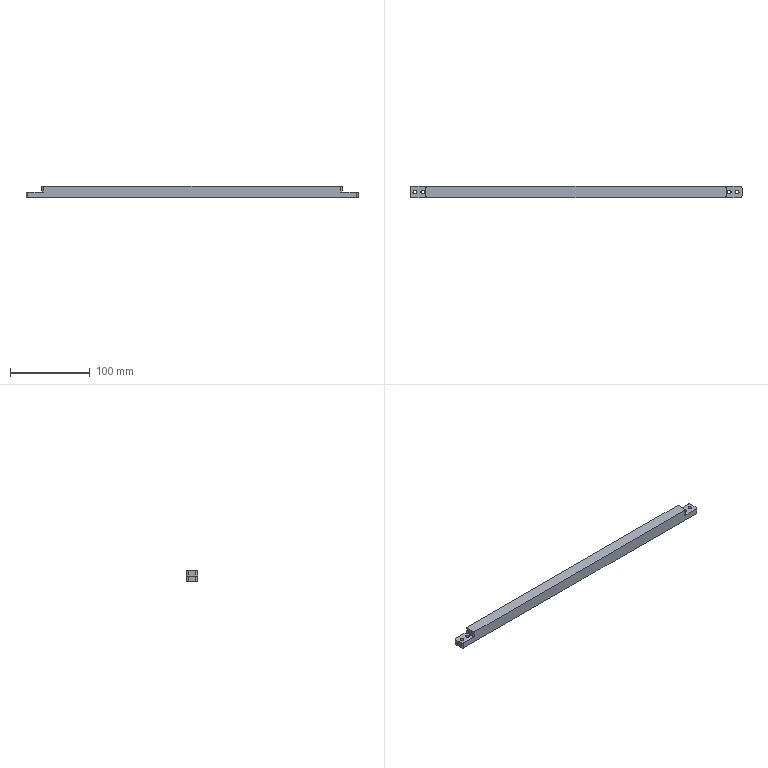Part | NX | 1 solid | 46 faces | box 417 x 14 x 15 mm | volume 81910 mm3 | cylinder 24 | plane 14 | cone 8 | commonest cylinder face diameters 2.459 x8 4 x8 4.5 x4 8 x4
STEP:
#1=CARTESIAN_POINT('',(-194.75,0.,-7.5));
#2=VERTEX_POINT('',#1);
#3=CARTESIAN_POINT('',(-192.5,0.,-7.5));
#4=DIRECTION('',(0.,0.,1.));
#5=DIRECTION('',(-1.,0.,0.));
#6=AXIS2_PLACEMENT_3D('',#3,#4,#5);
#7=CIRCLE('',#6,2.25);
#8=EDGE_CURVE('',#2,#2,#7,.T.);
#9=ORIENTED_EDGE('',*,*,#8,.T.);
#10=EDGE_LOOP('',(#9));
#11=FACE_BOUND('',#10,.T.);
#12=CARTESIAN_POINT('',(-194.75,0.,-10.5));
#13=VERTEX_POINT('',#12);
#14=CARTESIAN_POINT('',(-192.5,0.,-10.5));
#15=DIRECTION('',(0.,0.,1.));
#16=DIRECTION('',(-1.,0.,0.));
#17=AXIS2_PLACEMENT_3D('',#14,#15,#16);
#18=CIRCLE('',#17,2.25);
#19=EDGE_CURVE('',#13,#13,#18,.T.);
#20=ORIENTED_EDGE('',*,*,#19,.F.);
#21=EDGE_LOOP('',(#20));
#22=FACE_BOUND('',#21,.T.);
#23=CARTESIAN_POINT('',(-192.5,0.,-15.));
#24=DIRECTION('',(0.,0.,1.));
#25=DIRECTION('',(0.,-1.,0.));
#26=AXIS2_PLACEMENT_3D('',#23,#24,#25);
#27=CYLINDRICAL_SURFACE('',#26,2.25);
#28=ADVANCED_FACE('',(#11,#22),#27,.F.);
#29=CARTESIAN_POINT('',(-196.5,0.,-10.5));
#30=VERTEX_POINT('',#29);
#31=CARTESIAN_POINT('',(-192.5,0.,-10.5));
#32=DIRECTION('',(0.,0.,1.));
#33=DIRECTION('',(-1.,0.,0.));
#34=AXIS2_PLACEMENT_3D('',#31,#32,#33);
#35=CIRCLE('',#34,4.);
#36=EDGE_CURVE('',#30,#30,#35,.T.);
#37=ORIENTED_EDGE('',*,*,#36,.T.);
#38=EDGE_LOOP('',(#37));
#39=FACE_BOUND('',#38,.T.);
#40=CARTESIAN_POINT('',(-188.5,0.,-15.));
#41=VERTEX_POINT('',#40);
#42=CARTESIAN_POINT('',(-192.5,0.,-15.));
#43=DIRECTION('',(0.,0.,-1.));
#44=DIRECTION('',(1.,0.,0.));
#45=AXIS2_PLACEMENT_3D('',#42,#43,#44);
#46=CIRCLE('',#45,4.);
#47=EDGE_CURVE('',#41,#41,#46,.T.);
#48=ORIENTED_EDGE('',*,*,#47,.T.);
#49=EDGE_LOOP('',(#48));
#50=FACE_BOUND('',#49,.T.);
#51=CARTESIAN_POINT('',(-192.5,0.,-15.));
#52=DIRECTION('',(0.,0.,1.));
#53=DIRECTION('',(0.,-1.,0.));
#54=AXIS2_PLACEMENT_3D('',#51,#52,#53);
#55=CYLINDRICAL_SURFACE('',#54,4.);
#56=ADVANCED_FACE('',(#39,#50),#55,.F.);
#57=ORIENTED_EDGE('',*,*,#19,.T.);
#58=EDGE_LOOP('',(#57));
#59=FACE_BOUND('',#58,.T.);
#60=ORIENTED_EDGE('',*,*,#36,.F.);
#61=EDGE_LOOP('',(#60));
#62=FACE_BOUND('',#61,.T.);
#63=CARTESIAN_POINT('',(202.5,-2.25,-10.5));
#64=DIRECTION('',(0.,0.,1.));
#65=DIRECTION('',(0.,-1.,0.));
#66=AXIS2_PLACEMENT_3D('',#63,#64,#65);
#67=PLANE('',#66);
#68=ADVANCED_FACE('',(#59,#62),#67,.F.);
#69=CARTESIAN_POINT('',(-206.5,0.,-10.5));
#70=VERTEX_POINT('',#69);
#71=CARTESIAN_POINT('',(-202.5,0.,-10.5));
#72=DIRECTION('',(0.,0.,1.));
#73=DIRECTION('',(-1.,0.,0.));
#74=AXIS2_PLACEMENT_3D('',#71,#72,#73);
#75=CIRCLE('',#74,4.);
#76=EDGE_CURVE('',#70,#70,#75,.T.);
#77=ORIENTED_EDGE('',*,*,#76,.T.);
#78=EDGE_LOOP('',(#77));
#79=FACE_BOUND('',#78,.T.);
#80=CARTESIAN_POINT('',(-198.5,0.,-15.));
#81=VERTEX_POINT('',#80);
#82=CARTESIAN_POINT('',(-202.5,0.,-15.));
#83=DIRECTION('',(0.,0.,-1.));
#84=DIRECTION('',(1.,0.,0.));
#85=AXIS2_PLACEMENT_3D('',#82,#83,#84);
#86=CIRCLE('',#85,4.);
#87=EDGE_CURVE('',#81,#81,#86,.T.);
#88=ORIENTED_EDGE('',*,*,#87,.T.);
#89=EDGE_LOOP('',(#88));
#90=FACE_BOUND('',#89,.T.);
#91=CARTESIAN_POINT('',(-202.5,0.,-15.));
#92=DIRECTION('',(0.,0.,1.));
#93=DIRECTION('',(0.,-1.,0.));
#94=AXIS2_PLACEMENT_3D('',#91,#92,#93);
#95=CYLINDRICAL_SURFACE('',#94,4.);
#96=ADVANCED_FACE('',(#79,#90),#95,.F.);
#97=CARTESIAN_POINT('',(-206.5,-7.,-15.));
#98=VERTEX_POINT('',#97);
#99=CARTESIAN_POINT('',(-208.5,-5.,-15.));
#100=VERTEX_POINT('',#99);
#101=CARTESIAN_POINT('',(-206.5,-5.,-15.));
#102=DIRECTION('',(0.,0.,-1.));
#103=DIRECTION('',(1.,0.,0.));
#104=AXIS2_PLACEMENT_3D('',#101,#102,#103);
#105=CIRCLE('',#104,2.);
#106=EDGE_CURVE('',#98,#100,#105,.T.);
#107=ORIENTED_EDGE('',*,*,#106,.F.);
#108=CARTESIAN_POINT('',(-206.5,-7.,-7.5));
#109=VERTEX_POINT('',#108);
#110=CARTESIAN_POINT('',(-206.5,-7.,-11.25));
#111=DIRECTION('',(0.,0.,-1.));
#112=VECTOR('',#111,1000.);
#113=LINE('',#110,#112);
#114=EDGE_CURVE('',#109,#98,#113,.T.);
#115=ORIENTED_EDGE('',*,*,#114,.F.);
#116=CARTESIAN_POINT('',(-208.5,-5.,-7.5));
#117=VERTEX_POINT('',#116);
#118=CARTESIAN_POINT('',(-206.5,-5.,-7.5));
#119=DIRECTION('',(0.,0.,1.));
#120=DIRECTION('',(-1.,0.,0.));
#121=AXIS2_PLACEMENT_3D('',#118,#119,#120);
#122=CIRCLE('',#121,2.);
#123=EDGE_CURVE('',#117,#109,#122,.T.);
#124=ORIENTED_EDGE('',*,*,#123,.F.);
#125=CARTESIAN_POINT('',(-208.5,-5.,-11.25));
#126=DIRECTION('',(0.,0.,-1.));
#127=VECTOR('',#126,1000.);
#128=LINE('',#125,#127);
#129=EDGE_CURVE('',#117,#100,#128,.T.);
#130=ORIENTED_EDGE('',*,*,#129,.T.);
#131=EDGE_LOOP('',(#107,#115,#124,#130));
#132=FACE_BOUND('',#131,.T.);
#133=CARTESIAN_POINT('',(-206.5,-5.,-7.5));
#134=DIRECTION('',(0.,0.,-1.));
#135=DIRECTION('',(0.,-1.,0.));
#136=AXIS2_PLACEMENT_3D('',#133,#134,#135);
#137=CYLINDRICAL_SURFACE('',#136,2.);
#138=ADVANCED_FACE('',(#132),#137,.T.);
#139=CARTESIAN_POINT('',(-188.5,-5.,-7.5));
#140=VERTEX_POINT('',#139);
#141=CARTESIAN_POINT('',(-186.5,-7.,-7.5));
#142=VERTEX_POINT('',#141);
#143=CARTESIAN_POINT('',(-186.5,-5.,-7.5));
#144=DIRECTION('',(0.,0.,1.));
#145=DIRECTION('',(-1.,0.,0.));
#146=AXIS2_PLACEMENT_3D('',#143,#144,#145);
#147=CIRCLE('',#146,2.);
#148=EDGE_CURVE('',#140,#142,#147,.T.);
#149=ORIENTED_EDGE('',*,*,#148,.T.);
#150=CARTESIAN_POINT('',(-186.5,-7.,0.));
#151=VERTEX_POINT('',#150);
#152=CARTESIAN_POINT('',(-186.5,-7.,-3.75));
#153=DIRECTION('',(0.,0.,-1.));
#154=VECTOR('',#153,1000.);
#155=LINE('',#152,#154);
#156=EDGE_CURVE('',#151,#142,#155,.T.);
#157=ORIENTED_EDGE('',*,*,#156,.F.);
#158=CARTESIAN_POINT('',(-188.5,-5.,0.));
#159=VERTEX_POINT('',#158);
#160=CARTESIAN_POINT('',(-186.5,-5.,0.));
#161=DIRECTION('',(0.,0.,-1.));
#162=DIRECTION('',(1.,0.,0.));
#163=AXIS2_PLACEMENT_3D('',#160,#161,#162);
#164=CIRCLE('',#163,2.);
#165=EDGE_CURVE('',#151,#159,#164,.T.);
#166=ORIENTED_EDGE('',*,*,#165,.T.);
#167=CARTESIAN_POINT('',(-188.5,-5.,-3.75));
#168=DIRECTION('',(0.,0.,-1.));
#169=VECTOR('',#168,1000.);
#170=LINE('',#167,#169);
#171=EDGE_CURVE('',#159,#140,#170,.T.);
#172=ORIENTED_EDGE('',*,*,#171,.T.);
#173=EDGE_LOOP('',(#149,#157,#166,#172));
#174=FACE_BOUND('',#173,.T.);
#175=CARTESIAN_POINT('',(-186.5,-5.,-7.5));
#176=DIRECTION('',(0.,0.,-1.));
#177=DIRECTION('',(0.,-1.,0.));
#178=AXIS2_PLACEMENT_3D('',#175,#176,#177);
#179=CYLINDRICAL_SURFACE('',#178,2.);
#180=ADVANCED_FACE('',(#174),#179,.T.);
#181=CARTESIAN_POINT('',(-186.5,7.,-7.5));
#182=VERTEX_POINT('',#181);
#183=CARTESIAN_POINT('',(-188.5,5.,-7.5));
#184=VERTEX_POINT('',#183);
#185=CARTESIAN_POINT('',(-186.5,5.,-7.5));
#186=DIRECTION('',(0.,0.,1.));
#187=DIRECTION('',(-1.,0.,0.));
#188=AXIS2_PLACEMENT_3D('',#185,#186,#187);
#189=CIRCLE('',#188,2.);
#190=EDGE_CURVE('',#182,#184,#189,.T.);
#191=ORIENTED_EDGE('',*,*,#190,.T.);
#192=CARTESIAN_POINT('',(-188.5,5.,0.));
#193=VERTEX_POINT('',#192);
#194=CARTESIAN_POINT('',(-188.5,5.,-3.75));
#195=DIRECTION('',(0.,0.,-1.));
#196=VECTOR('',#195,1000.);
#197=LINE('',#194,#196);
#198=EDGE_CURVE('',#193,#184,#197,.T.);
#199=ORIENTED_EDGE('',*,*,#198,.F.);
#200=CARTESIAN_POINT('',(-186.5,7.,0.));
#201=VERTEX_POINT('',#200);
#202=CARTESIAN_POINT('',(-186.5,5.,0.));
#203=DIRECTION('',(0.,0.,-1.));
#204=DIRECTION('',(1.,0.,0.));
#205=AXIS2_PLACEMENT_3D('',#202,#203,#204);
#206=CIRCLE('',#205,2.);
#207=EDGE_CURVE('',#193,#201,#206,.T.);
#208=ORIENTED_EDGE('',*,*,#207,.T.);
#209=CARTESIAN_POINT('',(-186.5,7.,-3.75));
#210=DIRECTION('',(0.,0.,-1.));
#211=VECTOR('',#210,1000.);
#212=LINE('',#209,#211);
#213=EDGE_CURVE('',#201,#182,#212,.T.);
#214=ORIENTED_EDGE('',*,*,#213,.T.);
#215=EDGE_LOOP('',(#191,#199,#208,#214));
#216=FACE_BOUND('',#215,.T.);
#217=CARTESIAN_POINT('',(-186.5,5.,-7.5));
#218=DIRECTION('',(0.,0.,-1.));
#219=DIRECTION('',(-1.,0.,0.));
#220=AXIS2_PLACEMENT_3D('',#217,#218,#219);
#221=CYLINDRICAL_SURFACE('',#220,2.);
#222=ADVANCED_FACE('',(#216),#221,.T.);
#223=CARTESIAN_POINT('',(-208.5,5.,-15.));
#224=VERTEX_POINT('',#223);
#225=CARTESIAN_POINT('',(-206.5,7.,-15.));
#226=VERTEX_POINT('',#225);
#227=CARTESIAN_POINT('',(-206.5,5.,-15.));
#228=DIRECTION('',(0.,0.,-1.));
#229=DIRECTION('',(1.,0.,0.));
#230=AXIS2_PLACEMENT_3D('',#227,#228,#229);
#231=CIRCLE('',#230,2.);
#232=EDGE_CURVE('',#224,#226,#231,.T.);
#233=ORIENTED_EDGE('',*,*,#232,.F.);
#234=CARTESIAN_POINT('',(-208.5,5.,-7.5));
#235=VERTEX_POINT('',#234);
#236=CARTESIAN_POINT('',(-208.5,5.,-11.25));
#237=DIRECTION('',(0.,0.,-1.));
#238=VECTOR('',#237,1000.);
#239=LINE('',#236,#238);
#240=EDGE_CURVE('',#235,#224,#239,.T.);
#241=ORIENTED_EDGE('',*,*,#240,.F.);
#242=CARTESIAN_POINT('',(-206.5,7.,-7.5));
#243=VERTEX_POINT('',#242);
#244=CARTESIAN_POINT('',(-206.5,5.,-7.5));
#245=DIRECTION('',(0.,0.,1.));
#246=DIRECTION('',(-1.,0.,0.));
#247=AXIS2_PLACEMENT_3D('',#244,#245,#246);
#248=CIRCLE('',#247,2.);
#249=EDGE_CURVE('',#243,#235,#248,.T.);
#250=ORIENTED_EDGE('',*,*,#249,.F.);
#251=CARTESIAN_POINT('',(-206.5,7.,-11.25));
#252=DIRECTION('',(0.,0.,-1.));
#253=VECTOR('',#252,1000.);
#254=LINE('',#251,#253);
#255=EDGE_CURVE('',#243,#226,#254,.T.);
#256=ORIENTED_EDGE('',*,*,#255,.T.);
#257=EDGE_LOOP('',(#233,#241,#250,#256));
#258=FACE_BOUND('',#257,.T.);
#259=CARTESIAN_POINT('',(-206.5,5.,-7.5));
#260=DIRECTION('',(0.,0.,-1.));
#261=DIRECTION('',(-1.,0.,0.));
#262=AXIS2_PLACEMENT_3D('',#259,#260,#261);
#263=CYLINDRICAL_SURFACE('',#262,2.);
#264=ADVANCED_FACE('',(#258),#263,.T.);
#265=CARTESIAN_POINT('',(-174.23,0.,-15.));
#266=VERTEX_POINT('',#265);
#267=CARTESIAN_POINT('',(-173.,0.,-15.));
#268=DIRECTION('',(0.,0.,1.));
#269=DIRECTION('',(-1.,0.,0.));
#270=AXIS2_PLACEMENT_3D('',#267,#268,#269);
#271=CIRCLE('',#270,1.23);
#272=EDGE_CURVE('',#266,#266,#271,.T.);
#273=ORIENTED_EDGE('',*,*,#272,.T.);
#274=EDGE_LOOP('',(#273));
#275=FACE_BOUND('',#274,.T.);
#276=CARTESIAN_POINT('',(-124.23,0.,-15.));
#277=VERTEX_POINT('',#276);
#278=CARTESIAN_POINT('',(-123.,0.,-15.));
#279=DIRECTION('',(0.,0.,1.));
#280=DIRECTION('',(-1.,0.,0.));
#281=AXIS2_PLACEMENT_3D('',#278,#279,#280);
#282=CIRCLE('',#281,1.23);
#283=EDGE_CURVE('',#277,#277,#282,.T.);
#284=ORIENTED_EDGE('',*,*,#283,.T.);
#285=EDGE_LOOP('',(#284));
#286=FACE_BOUND('',#285,.T.);
#287=CARTESIAN_POINT('',(-74.23,0.,-15.));
#288=VERTEX_POINT('',#287);
#289=CARTESIAN_POINT('',(-73.,0.,-15.));
#290=DIRECTION('',(0.,0.,1.));
#291=DIRECTION('',(-1.,0.,0.));
#292=AXIS2_PLACEMENT_3D('',#289,#290,#291);
#293=CIRCLE('',#292,1.23);
#294=EDGE_CURVE('',#288,#288,#293,.T.);
#295=ORIENTED_EDGE('',*,*,#294,.T.);
#296=EDGE_LOOP('',(#295));
#297=FACE_BOUND('',#296,.T.);
#298=CARTESIAN_POINT('',(-24.23,0.,-15.));
#299=VERTEX_POINT('',#298);
#300=CARTESIAN_POINT('',(-23.,0.,-15.));
#301=DIRECTION('',(0.,0.,1.));
#302=DIRECTION('',(-1.,0.,0.));
#303=AXIS2_PLACEMENT_3D('',#300,#301,#302);
#304=CIRCLE('',#303,1.23);
#305=EDGE_CURVE('',#299,#299,#304,.T.);
#306=ORIENTED_EDGE('',*,*,#305,.T.);
#307=EDGE_LOOP('',(#306));
#308=FACE_BOUND('',#307,.T.);
#309=CARTESIAN_POINT('',(25.77,0.,-15.));
#310=VERTEX_POINT('',#309);
#311=CARTESIAN_POINT('',(27.,0.,-15.));
#312=DIRECTION('',(0.,0.,1.));
#313=DIRECTION('',(-1.,0.,0.));
#314=AXIS2_PLACEMENT_3D('',#311,#312,#313);
#315=CIRCLE('',#314,1.23);
#316=EDGE_CURVE('',#310,#310,#315,.T.);
#317=ORIENTED_EDGE('',*,*,#316,.T.);
#318=EDGE_LOOP('',(#317));
#319=FACE_BOUND('',#318,.T.);
#320=CARTESIAN_POINT('',(75.77,0.,-15.));
#321=VERTEX_POINT('',#320);
#322=CARTESIAN_POINT('',(77.,0.,-15.));
#323=DIRECTION('',(0.,0.,1.));
#324=DIRECTION('',(-1.,0.,0.));
#325=AXIS2_PLACEMENT_3D('',#322,#323,#324);
#326=CIRCLE('',#325,1.23);
#327=EDGE_CURVE('',#321,#321,#326,.T.);
#328=ORIENTED_EDGE('',*,*,#327,.T.);
#329=EDGE_LOOP('',(#328));
#330=FACE_BOUND('',#329,.T.);
#331=CARTESIAN_POINT('',(125.77,0.,-15.));
#332=VERTEX_POINT('',#331);
#333=CARTESIAN_POINT('',(127.,0.,-15.));
#334=DIRECTION('',(0.,0.,1.));
#335=DIRECTION('',(-1.,0.,0.));
#336=AXIS2_PLACEMENT_3D('',#333,#334,#335);
#337=CIRCLE('',#336,1.23);
#338=EDGE_CURVE('',#332,#332,#337,.T.);
#339=ORIENTED_EDGE('',*,*,#338,.T.);
#340=EDGE_LOOP('',(#339));
#341=FACE_BOUND('',#340,.T.);
#342=CARTESIAN_POINT('',(198.5,0.,-15.));
#343=VERTEX_POINT('',#342);
#344=CARTESIAN_POINT('',(202.5,0.,-15.));
#345=DIRECTION('',(0.,0.,1.));
#346=DIRECTION('',(-1.,0.,0.));
#347=AXIS2_PLACEMENT_3D('',#344,#345,#346);
#348=CIRCLE('',#347,4.);
#349=EDGE_CURVE('',#343,#343,#348,.T.);
#350=ORIENTED_EDGE('',*,*,#349,.T.);
#351=EDGE_LOOP('',(#350));
#352=FACE_BOUND('',#351,.T.);
#353=CARTESIAN_POINT('',(188.5,0.,-15.));
#354=VERTEX_POINT('',#353);
#355=CARTESIAN_POINT('',(192.5,0.,-15.));
#356=DIRECTION('',(0.,0.,1.));
#357=DIRECTION('',(-1.,0.,0.));
#358=AXIS2_PLACEMENT_3D('',#355,#356,#357);
#359=CIRCLE('',#358,4.);
#360=EDGE_CURVE('',#354,#354,#359,.T.);
#361=ORIENTED_EDGE('',*,*,#360,.T.);
#362=EDGE_LOOP('',(#361));
#363=FACE_BOUND('',#362,.T.);
#364=CARTESIAN_POINT('',(175.77,0.,-15.));
#365=VERTEX_POINT('',#364);
#366=CARTESIAN_POINT('',(177.,0.,-15.));
#367=DIRECTION('',(0.,0.,1.));
#368=DIRECTION('',(-1.,0.,0.));
#369=AXIS2_PLACEMENT_3D('',#366,#367,#368);
#370=CIRCLE('',#369,1.23);
#371=EDGE_CURVE('',#365,#365,#370,.T.);
#372=ORIENTED_EDGE('',*,*,#371,.T.);
#373=EDGE_LOOP('',(#372));
#374=FACE_BOUND('',#373,.T.);
#375=ORIENTED_EDGE('',*,*,#87,.F.);
#376=EDGE_LOOP('',(#375));
#377=FACE_BOUND('',#376,.T.);
#378=ORIENTED_EDGE('',*,*,#47,.F.);
#379=EDGE_LOOP('',(#378));
#380=FACE_BOUND('',#379,.T.);
#381=CARTESIAN_POINT('',(206.5,7.,-15.));
#382=VERTEX_POINT('',#381);
#383=CARTESIAN_POINT('',(0.,7.,-15.));
#384=DIRECTION('',(-1.,0.,0.));
#385=VECTOR('',#384,1000.);
#386=LINE('',#383,#385);
#387=EDGE_CURVE('',#382,#226,#386,.T.);
#388=ORIENTED_EDGE('',*,*,#387,.F.);
#389=CARTESIAN_POINT('',(208.5,5.,-15.));
#390=VERTEX_POINT('',#389);
#391=CARTESIAN_POINT('',(206.5,5.,-15.));
#392=DIRECTION('',(0.,0.,-1.));
#393=DIRECTION('',(1.,0.,0.));
#394=AXIS2_PLACEMENT_3D('',#391,#392,#393);
#395=CIRCLE('',#394,2.);
#396=EDGE_CURVE('',#382,#390,#395,.T.);
#397=ORIENTED_EDGE('',*,*,#396,.T.);
#398=CARTESIAN_POINT('',(208.5,-5.,-15.));
#399=VERTEX_POINT('',#398);
#400=CARTESIAN_POINT('',(208.5,0.,-15.));
#401=DIRECTION('',(0.,-1.,0.));
#402=VECTOR('',#401,1000.);
#403=LINE('',#400,#402);
#404=EDGE_CURVE('',#390,#399,#403,.T.);
#405=ORIENTED_EDGE('',*,*,#404,.T.);
#406=CARTESIAN_POINT('',(206.5,-7.,-15.));
#407=VERTEX_POINT('',#406);
#408=CARTESIAN_POINT('',(206.5,-5.,-15.));
#409=DIRECTION('',(0.,0.,-1.));
#410=DIRECTION('',(1.,0.,0.));
#411=AXIS2_PLACEMENT_3D('',#408,#409,#410);
#412=CIRCLE('',#411,2.);
#413=EDGE_CURVE('',#399,#407,#412,.T.);
#414=ORIENTED_EDGE('',*,*,#413,.T.);
#415=CARTESIAN_POINT('',(0.,-7.,-15.));
#416=DIRECTION('',(1.,0.,0.));
#417=VECTOR('',#416,1000.);
#418=LINE('',#415,#417);
#419=EDGE_CURVE('',#98,#407,#418,.T.);
#420=ORIENTED_EDGE('',*,*,#419,.F.);
#421=ORIENTED_EDGE('',*,*,#106,.T.);
#422=CARTESIAN_POINT('',(-208.5,0.,-15.));
#423=DIRECTION('',(0.,1.,0.));
#424=VECTOR('',#423,1000.);
#425=LINE('',#422,#424);
#426=EDGE_CURVE('',#100,#224,#425,.T.);
#427=ORIENTED_EDGE('',*,*,#426,.T.);
#428=ORIENTED_EDGE('',*,*,#232,.T.);
#429=EDGE_LOOP('',(#388,#397,#405,#414,#420,#421,#427,#428));
#430=FACE_BOUND('',#429,.T.);
#431=CARTESIAN_POINT('',(208.5,-7.,-15.));
#432=DIRECTION('',(0.,0.,-1.));
#433=DIRECTION('',(0.,-1.,0.));
#434=AXIS2_PLACEMENT_3D('',#431,#432,#433);
#435=PLANE('',#434);
#436=ADVANCED_FACE('',(#275,#286,#297,#308,#319,#330,#341,#352,#363,#374,#377,#380,#430),#435,.T.);
#437=CARTESIAN_POINT('',(186.5,-7.,-7.5));
#438=VERTEX_POINT('',#437);
#439=CARTESIAN_POINT('',(188.5,-5.,-7.5));
#440=VERTEX_POINT('',#439);
#441=CARTESIAN_POINT('',(186.5,-5.,-7.5));
#442=DIRECTION('',(0.,0.,1.));
#443=DIRECTION('',(-1.,0.,0.));
#444=AXIS2_PLACEMENT_3D('',#441,#442,#443);
#445=CIRCLE('',#444,2.);
#446=EDGE_CURVE('',#438,#440,#445,.T.);
#447=ORIENTED_EDGE('',*,*,#446,.T.);
#448=CARTESIAN_POINT('',(188.5,-5.,0.));
#449=VERTEX_POINT('',#448);
#450=CARTESIAN_POINT('',(188.5,-5.,-3.75));
#451=DIRECTION('',(0.,0.,-1.));
#452=VECTOR('',#451,1000.);
#453=LINE('',#450,#452);
#454=EDGE_CURVE('',#449,#440,#453,.T.);
#455=ORIENTED_EDGE('',*,*,#454,.F.);
#456=CARTESIAN_POINT('',(186.5,-7.,0.));
#457=VERTEX_POINT('',#456);
#458=CARTESIAN_POINT('',(186.5,-5.,0.));
#459=DIRECTION('',(0.,0.,-1.));
#460=DIRECTION('',(1.,0.,0.));
#461=AXIS2_PLACEMENT_3D('',#458,#459,#460);
#462=CIRCLE('',#461,2.);
#463=EDGE_CURVE('',#449,#457,#462,.T.);
#464=ORIENTED_EDGE('',*,*,#463,.T.);
#465=CARTESIAN_POINT('',(186.5,-7.,-3.75));
#466=DIRECTION('',(0.,0.,-1.));
#467=VECTOR('',#466,1000.);
#468=LINE('',#465,#467);
#469=EDGE_CURVE('',#457,#438,#468,.T.);
#470=ORIENTED_EDGE('',*,*,#469,.T.);
#471=EDGE_LOOP('',(#447,#455,#464,#470));
#472=FACE_BOUND('',#471,.T.);
#473=CARTESIAN_POINT('',(186.5,-5.,-7.5));
#474=DIRECTION('',(0.,0.,-1.));
#475=DIRECTION('',(1.,0.,0.));
#476=AXIS2_PLACEMENT_3D('',#473,#474,#475);
#477=CYLINDRICAL_SURFACE('',#476,2.);
#478=ADVANCED_FACE('',(#472),#477,.T.);
#479=CARTESIAN_POINT('',(200.25,0.,-7.5));
#480=VERTEX_POINT('',#479);
#481=CARTESIAN_POINT('',(202.5,0.,-7.5));
#482=DIRECTION('',(0.,0.,1.));
#483=DIRECTION('',(-1.,0.,0.));
#484=AXIS2_PLACEMENT_3D('',#481,#482,#483);
#485=CIRCLE('',#484,2.25);
#486=EDGE_CURVE('',#480,#480,#485,.T.);
#487=ORIENTED_EDGE('',*,*,#486,.F.);
#488=EDGE_LOOP('',(#487));
#489=FACE_BOUND('',#488,.T.);
#490=CARTESIAN_POINT('',(190.25,0.,-7.5));
#491=VERTEX_POINT('',#490);
#492=CARTESIAN_POINT('',(192.5,0.,-7.5));
#493=DIRECTION('',(0.,0.,1.));
#494=DIRECTION('',(-1.,0.,0.));
#495=AXIS2_PLACEMENT_3D('',#492,#493,#494);
#496=CIRCLE('',#495,2.25);
#497=EDGE_CURVE('',#491,#491,#496,.T.);
#498=ORIENTED_EDGE('',*,*,#497,.F.);
#499=EDGE_LOOP('',(#498));
#500=FACE_BOUND('',#499,.T.);
#501=CARTESIAN_POINT('',(186.5,7.,-7.5));
#502=VERTEX_POINT('',#501);
#503=CARTESIAN_POINT('',(206.5,7.,-7.5));
#504=VERTEX_POINT('',#503);
#505=CARTESIAN_POINT('',(196.5,7.,-7.5));
#506=DIRECTION('',(1.,0.,0.));
#507=VECTOR('',#506,1000.);
#508=LINE('',#505,#507);
#509=EDGE_CURVE('',#502,#504,#508,.T.);
#510=ORIENTED_EDGE('',*,*,#509,.F.);
#511=CARTESIAN_POINT('',(188.5,5.,-7.5));
#512=VERTEX_POINT('',#511);
#513=CARTESIAN_POINT('',(186.5,5.,-7.5));
#514=DIRECTION('',(0.,0.,-1.));
#515=DIRECTION('',(1.,0.,0.));
#516=AXIS2_PLACEMENT_3D('',#513,#514,#515);
#517=CIRCLE('',#516,2.);
#518=EDGE_CURVE('',#502,#512,#517,.T.);
#519=ORIENTED_EDGE('',*,*,#518,.T.);
#520=CARTESIAN_POINT('',(188.5,0.,-7.5));
#521=DIRECTION('',(0.,-1.,0.));
#522=VECTOR('',#521,1000.);
#523=LINE('',#520,#522);
#524=EDGE_CURVE('',#512,#440,#523,.T.);
#525=ORIENTED_EDGE('',*,*,#524,.T.);
#526=ORIENTED_EDGE('',*,*,#446,.F.);
#527=CARTESIAN_POINT('',(206.5,-7.,-7.5));
#528=VERTEX_POINT('',#527);
#529=CARTESIAN_POINT('',(196.5,-7.,-7.5));
#530=DIRECTION('',(-1.,0.,0.));
#531=VECTOR('',#530,1000.);
#532=LINE('',#529,#531);
#533=EDGE_CURVE('',#528,#438,#532,.T.);
#534=ORIENTED_EDGE('',*,*,#533,.F.);
#535=CARTESIAN_POINT('',(208.5,-5.,-7.5));
#536=VERTEX_POINT('',#535);
#537=CARTESIAN_POINT('',(206.5,-5.,-7.5));
#538=DIRECTION('',(0.,0.,-1.));
#539=DIRECTION('',(1.,0.,0.));
#540=AXIS2_PLACEMENT_3D('',#537,#538,#539);
#541=CIRCLE('',#540,2.);
#542=EDGE_CURVE('',#536,#528,#541,.T.);
#543=ORIENTED_EDGE('',*,*,#542,.F.);
#544=CARTESIAN_POINT('',(208.5,5.,-7.5));
#545=VERTEX_POINT('',#544);
#546=CARTESIAN_POINT('',(208.5,0.,-7.5));
#547=DIRECTION('',(0.,1.,0.));
#548=VECTOR('',#547,1000.);
#549=LINE('',#546,#548);
#550=EDGE_CURVE('',#536,#545,#549,.T.);
#551=ORIENTED_EDGE('',*,*,#550,.T.);
#552=CARTESIAN_POINT('',(206.5,5.,-7.5));
#553=DIRECTION('',(0.,0.,-1.));
#554=DIRECTION('',(1.,0.,0.));
#555=AXIS2_PLACEMENT_3D('',#552,#553,#554);
#556=CIRCLE('',#555,2.);
#557=EDGE_CURVE('',#504,#545,#556,.T.);
#558=ORIENTED_EDGE('',*,*,#557,.F.);
#559=EDGE_LOOP('',(#510,#519,#525,#526,#534,#543,#551,#558));
#560=FACE_BOUND('',#559,.T.);
#561=CARTESIAN_POINT('',(208.5,-7.,-7.5));
#562=DIRECTION('',(0.,0.,1.));
#563=DIRECTION('',(0.,1.,0.));
#564=AXIS2_PLACEMENT_3D('',#561,#562,#563);
#565=PLANE('',#564);
#566=ADVANCED_FACE('',(#489,#500,#560),#565,.T.);
#567=ORIENTED_EDGE('',*,*,#413,.F.);
#568=CARTESIAN_POINT('',(208.5,-5.,-11.25));
#569=DIRECTION('',(0.,0.,-1.));
#570=VECTOR('',#569,1000.);
#571=LINE('',#568,#570);
#572=EDGE_CURVE('',#536,#399,#571,.T.);
#573=ORIENTED_EDGE('',*,*,#572,.F.);
#574=ORIENTED_EDGE('',*,*,#542,.T.);
#575=CARTESIAN_POINT('',(206.5,-7.,-11.25));
#576=DIRECTION('',(0.,0.,-1.));
#577=VECTOR('',#576,1000.);
#578=LINE('',#575,#577);
#579=EDGE_CURVE('',#528,#407,#578,.T.);
#580=ORIENTED_EDGE('',*,*,#579,.T.);
#581=EDGE_LOOP('',(#567,#573,#574,#580));
#582=FACE_BOUND('',#581,.T.);
#583=CARTESIAN_POINT('',(206.5,-5.,-7.5));
#584=DIRECTION('',(0.,0.,-1.));
#585=DIRECTION('',(1.,0.,0.));
#586=AXIS2_PLACEMENT_3D('',#583,#584,#585);
#587=CYLINDRICAL_SURFACE('',#586,2.);
#588=ADVANCED_FACE('',(#582),#587,.T.);
#589=CARTESIAN_POINT('',(188.5,5.,0.));
#590=VERTEX_POINT('',#589);
#591=CARTESIAN_POINT('',(188.5,0.,0.));
#592=DIRECTION('',(0.,-1.,0.));
#593=VECTOR('',#592,1000.);
#594=LINE('',#591,#593);
#595=EDGE_CURVE('',#590,#449,#594,.T.);
#596=ORIENTED_EDGE('',*,*,#595,.T.);
#597=ORIENTED_EDGE('',*,*,#454,.T.);
#598=ORIENTED_EDGE('',*,*,#524,.F.);
#599=CARTESIAN_POINT('',(188.5,5.,-7.5));
#600=DIRECTION('',(0.,0.,-1.));
#601=VECTOR('',#600,1000.);
#602=LINE('',#599,#601);
#603=EDGE_CURVE('',#590,#512,#602,.T.);
#604=ORIENTED_EDGE('',*,*,#603,.F.);
#605=EDGE_LOOP('',(#596,#597,#598,#604));
#606=FACE_BOUND('',#605,.T.);
#607=CARTESIAN_POINT('',(188.5,7.,0.));
#608=DIRECTION('',(1.,0.,0.));
#609=DIRECTION('',(0.,-1.,0.));
#610=AXIS2_PLACEMENT_3D('',#607,#608,#609);
#611=PLANE('',#610);
#612=ADVANCED_FACE('',(#606),#611,.T.);
#613=CARTESIAN_POINT('',(178.23,0.,-7.));
#614=VERTEX_POINT('',#613);
#615=CARTESIAN_POINT('',(177.,0.,-7.));
#616=DIRECTION('',(0.,0.,-1.));
#617=DIRECTION('',(1.,0.,0.));
#618=AXIS2_PLACEMENT_3D('',#615,#616,#617);
#619=CIRCLE('',#618,1.23);
#620=EDGE_CURVE('',#614,#614,#619,.T.);
#621=ORIENTED_EDGE('',*,*,#620,.F.);
#622=EDGE_LOOP('',(#621));
#623=FACE_BOUND('',#622,.T.);
#624=ORIENTED_EDGE('',*,*,#371,.F.);
#625=EDGE_LOOP('',(#624));
#626=FACE_BOUND('',#625,.T.);
#627=CARTESIAN_POINT('',(177.,0.,-15.));
#628=DIRECTION('',(0.,0.,1.));
#629=DIRECTION('',(0.,-1.,0.));
#630=AXIS2_PLACEMENT_3D('',#627,#628,#629);
#631=CYLINDRICAL_SURFACE('',#630,1.23);
#632=ADVANCED_FACE('',(#623,#626),#631,.F.);
#633=CARTESIAN_POINT('',(188.5,0.,-10.5));
#634=VERTEX_POINT('',#633);
#635=CARTESIAN_POINT('',(192.5,0.,-10.5));
#636=DIRECTION('',(0.,0.,1.));
#637=DIRECTION('',(-1.,0.,0.));
#638=AXIS2_PLACEMENT_3D('',#635,#636,#637);
#639=CIRCLE('',#638,4.);
#640=EDGE_CURVE('',#634,#634,#639,.T.);
#641=ORIENTED_EDGE('',*,*,#640,.T.);
#642=EDGE_LOOP('',(#641));
#643=FACE_BOUND('',#642,.T.);
#644=ORIENTED_EDGE('',*,*,#360,.F.);
#645=EDGE_LOOP('',(#644));
#646=FACE_BOUND('',#645,.T.);
#647=CARTESIAN_POINT('',(192.5,0.,-15.));
#648=DIRECTION('',(0.,0.,1.));
#649=DIRECTION('',(0.,-1.,0.));
#650=AXIS2_PLACEMENT_3D('',#647,#648,#649);
#651=CYLINDRICAL_SURFACE('',#650,4.);
#652=ADVANCED_FACE('',(#643,#646),#651,.F.);
#653=CARTESIAN_POINT('',(198.5,0.,-10.5));
#654=VERTEX_POINT('',#653);
#655=CARTESIAN_POINT('',(202.5,0.,-10.5));
#656=DIRECTION('',(0.,0.,1.));
#657=DIRECTION('',(-1.,0.,0.));
#658=AXIS2_PLACEMENT_3D('',#655,#656,#657);
#659=CIRCLE('',#658,4.);
#660=EDGE_CURVE('',#654,#654,#659,.T.);
#661=ORIENTED_EDGE('',*,*,#660,.T.);
#662=EDGE_LOOP('',(#661));
#663=FACE_BOUND('',#662,.T.);
#664=ORIENTED_EDGE('',*,*,#349,.F.);
#665=EDGE_LOOP('',(#664));
#666=FACE_BOUND('',#665,.T.);
#667=CARTESIAN_POINT('',(202.5,0.,-15.));
#668=DIRECTION('',(0.,0.,1.));
#669=DIRECTION('',(0.,-1.,0.));
#670=AXIS2_PLACEMENT_3D('',#667,#668,#669);
#671=CYLINDRICAL_SURFACE('',#670,4.);
#672=ADVANCED_FACE('',(#663,#666),#671,.F.);
#673=CARTESIAN_POINT('',(128.23,0.,-7.));
#674=VERTEX_POINT('',#673);
#675=CARTESIAN_POINT('',(127.,0.,-7.));
#676=DIRECTION('',(0.,0.,-1.));
#677=DIRECTION('',(1.,0.,0.));
#678=AXIS2_PLACEMENT_3D('',#675,#676,#677);
#679=CIRCLE('',#678,1.23);
#680=EDGE_CURVE('',#674,#674,#679,.T.);
#681=ORIENTED_EDGE('',*,*,#680,.F.);
#682=EDGE_LOOP('',(#681));
#683=FACE_BOUND('',#682,.T.);
#684=ORIENTED_EDGE('',*,*,#338,.F.);
#685=EDGE_LOOP('',(#684));
#686=FACE_BOUND('',#685,.T.);
#687=CARTESIAN_POINT('',(127.,0.,-15.));
#688=DIRECTION('',(0.,0.,1.));
#689=DIRECTION('',(0.,-1.,0.));
#690=AXIS2_PLACEMENT_3D('',#687,#688,#689);
#691=CYLINDRICAL_SURFACE('',#690,1.23);
#692=ADVANCED_FACE('',(#683,#686),#691,.F.);
#693=CARTESIAN_POINT('',(78.23,0.,-7.));
#694=VERTEX_POINT('',#693);
#695=CARTESIAN_POINT('',(77.,0.,-7.));
#696=DIRECTION('',(0.,0.,-1.));
#697=DIRECTION('',(1.,0.,0.));
#698=AXIS2_PLACEMENT_3D('',#695,#696,#697);
#699=CIRCLE('',#698,1.23);
#700=EDGE_CURVE('',#694,#694,#699,.T.);
#701=ORIENTED_EDGE('',*,*,#700,.F.);
#702=EDGE_LOOP('',(#701));
#703=FACE_BOUND('',#702,.T.);
#704=ORIENTED_EDGE('',*,*,#327,.F.);
#705=EDGE_LOOP('',(#704));
#706=FACE_BOUND('',#705,.T.);
#707=CARTESIAN_POINT('',(77.,0.,-15.));
#708=DIRECTION('',(0.,0.,1.));
#709=DIRECTION('',(0.,-1.,0.));
#710=AXIS2_PLACEMENT_3D('',#707,#708,#709);
#711=CYLINDRICAL_SURFACE('',#710,1.23);
#712=ADVANCED_FACE('',(#703,#706),#711,.F.);
#713=CARTESIAN_POINT('',(28.23,0.,-7.));
#714=VERTEX_POINT('',#713);
#715=CARTESIAN_POINT('',(27.,0.,-7.));
#716=DIRECTION('',(0.,0.,-1.));
#717=DIRECTION('',(1.,0.,0.));
#718=AXIS2_PLACEMENT_3D('',#715,#716,#717);
#719=CIRCLE('',#718,1.23);
#720=EDGE_CURVE('',#714,#714,#719,.T.);
#721=ORIENTED_EDGE('',*,*,#720,.F.);
#722=EDGE_LOOP('',(#721));
#723=FACE_BOUND('',#722,.T.);
#724=ORIENTED_EDGE('',*,*,#316,.F.);
#725=EDGE_LOOP('',(#724));
#726=FACE_BOUND('',#725,.T.);
#727=CARTESIAN_POINT('',(27.,0.,-15.));
#728=DIRECTION('',(0.,0.,1.));
#729=DIRECTION('',(0.,-1.,0.));
#730=AXIS2_PLACEMENT_3D('',#727,#728,#729);
#731=CYLINDRICAL_SURFACE('',#730,1.23);
#732=ADVANCED_FACE('',(#723,#726),#731,.F.);
#733=CARTESIAN_POINT('',(-21.77,0.,-7.));
#734=VERTEX_POINT('',#733);
#735=CARTESIAN_POINT('',(-23.,0.,-7.));
#736=DIRECTION('',(0.,0.,-1.));
#737=DIRECTION('',(1.,0.,0.));
#738=AXIS2_PLACEMENT_3D('',#735,#736,#737);
#739=CIRCLE('',#738,1.23);
#740=EDGE_CURVE('',#734,#734,#739,.T.);
#741=ORIENTED_EDGE('',*,*,#740,.F.);
#742=EDGE_LOOP('',(#741));
#743=FACE_BOUND('',#742,.T.);
#744=ORIENTED_EDGE('',*,*,#305,.F.);
#745=EDGE_LOOP('',(#744));
#746=FACE_BOUND('',#745,.T.);
#747=CARTESIAN_POINT('',(-23.,0.,-15.));
#748=DIRECTION('',(0.,0.,1.));
#749=DIRECTION('',(0.,-1.,0.));
#750=AXIS2_PLACEMENT_3D('',#747,#748,#749);
#751=CYLINDRICAL_SURFACE('',#750,1.23);
#752=ADVANCED_FACE('',(#743,#746),#751,.F.);
#753=CARTESIAN_POINT('',(-71.77,0.,-7.));
#754=VERTEX_POINT('',#753);
#755=CARTESIAN_POINT('',(-73.,0.,-7.));
#756=DIRECTION('',(0.,0.,-1.));
#757=DIRECTION('',(1.,0.,0.));
#758=AXIS2_PLACEMENT_3D('',#755,#756,#757);
#759=CIRCLE('',#758,1.23);
#760=EDGE_CURVE('',#754,#754,#759,.T.);
#761=ORIENTED_EDGE('',*,*,#760,.F.);
#762=EDGE_LOOP('',(#761));
#763=FACE_BOUND('',#762,.T.);
#764=ORIENTED_EDGE('',*,*,#294,.F.);
#765=EDGE_LOOP('',(#764));
#766=FACE_BOUND('',#765,.T.);
#767=CARTESIAN_POINT('',(-73.,0.,-15.));
#768=DIRECTION('',(0.,0.,1.));
#769=DIRECTION('',(0.,-1.,0.));
#770=AXIS2_PLACEMENT_3D('',#767,#768,#769);
#771=CYLINDRICAL_SURFACE('',#770,1.23);
#772=ADVANCED_FACE('',(#763,#766),#771,.F.);
#773=CARTESIAN_POINT('',(-121.77,0.,-7.));
#774=VERTEX_POINT('',#773);
#775=CARTESIAN_POINT('',(-123.,0.,-7.));
#776=DIRECTION('',(0.,0.,-1.));
#777=DIRECTION('',(1.,0.,0.));
#778=AXIS2_PLACEMENT_3D('',#775,#776,#777);
#779=CIRCLE('',#778,1.23);
#780=EDGE_CURVE('',#774,#774,#779,.T.);
#781=ORIENTED_EDGE('',*,*,#780,.F.);
#782=EDGE_LOOP('',(#781));
#783=FACE_BOUND('',#782,.T.);
#784=ORIENTED_EDGE('',*,*,#283,.F.);
#785=EDGE_LOOP('',(#784));
#786=FACE_BOUND('',#785,.T.);
#787=CARTESIAN_POINT('',(-123.,0.,-15.));
#788=DIRECTION('',(0.,0.,1.));
#789=DIRECTION('',(0.,-1.,0.));
#790=AXIS2_PLACEMENT_3D('',#787,#788,#789);
#791=CYLINDRICAL_SURFACE('',#790,1.23);
#792=ADVANCED_FACE('',(#783,#786),#791,.F.);
#793=CARTESIAN_POINT('',(-171.77,0.,-7.));
#794=VERTEX_POINT('',#793);
#795=CARTESIAN_POINT('',(-173.,0.,-7.));
#796=DIRECTION('',(0.,0.,-1.));
#797=DIRECTION('',(1.,0.,0.));
#798=AXIS2_PLACEMENT_3D('',#795,#796,#797);
#799=CIRCLE('',#798,1.23);
#800=EDGE_CURVE('',#794,#794,#799,.T.);
#801=ORIENTED_EDGE('',*,*,#800,.F.);
#802=EDGE_LOOP('',(#801));
#803=FACE_BOUND('',#802,.T.);
#804=ORIENTED_EDGE('',*,*,#272,.F.);
#805=EDGE_LOOP('',(#804));
#806=FACE_BOUND('',#805,.T.);
#807=CARTESIAN_POINT('',(-173.,0.,-15.));
#808=DIRECTION('',(0.,0.,1.));
#809=DIRECTION('',(0.,-1.,0.));
#810=AXIS2_PLACEMENT_3D('',#807,#808,#809);
#811=CYLINDRICAL_SURFACE('',#810,1.23);
#812=ADVANCED_FACE('',(#803,#806),#811,.F.);
#813=ORIENTED_EDGE('',*,*,#497,.T.);
#814=EDGE_LOOP('',(#813));
#815=FACE_BOUND('',#814,.T.);
#816=CARTESIAN_POINT('',(190.25,0.,-10.5));
#817=VERTEX_POINT('',#816);
#818=CARTESIAN_POINT('',(192.5,0.,-10.5));
#819=DIRECTION('',(0.,0.,1.));
#820=DIRECTION('',(-1.,0.,0.));
#821=AXIS2_PLACEMENT_3D('',#818,#819,#820);
#822=CIRCLE('',#821,2.25);
#823=EDGE_CURVE('',#817,#817,#822,.T.);
#824=ORIENTED_EDGE('',*,*,#823,.F.);
#825=EDGE_LOOP('',(#824));
#826=FACE_BOUND('',#825,.T.);
#827=CARTESIAN_POINT('',(192.5,0.,-15.));
#828=DIRECTION('',(0.,0.,1.));
#829=DIRECTION('',(0.,-1.,0.));
#830=AXIS2_PLACEMENT_3D('',#827,#828,#829);
#831=CYLINDRICAL_SURFACE('',#830,2.25);
#832=ADVANCED_FACE('',(#815,#826),#831,.F.);
#833=ORIENTED_EDGE('',*,*,#486,.T.);
#834=EDGE_LOOP('',(#833));
#835=FACE_BOUND('',#834,.T.);
#836=CARTESIAN_POINT('',(200.25,0.,-10.5));
#837=VERTEX_POINT('',#836);
#838=CARTESIAN_POINT('',(202.5,0.,-10.5));
#839=DIRECTION('',(0.,0.,1.));
#840=DIRECTION('',(-1.,0.,0.));
#841=AXIS2_PLACEMENT_3D('',#838,#839,#840);
#842=CIRCLE('',#841,2.25);
#843=EDGE_CURVE('',#837,#837,#842,.T.);
#844=ORIENTED_EDGE('',*,*,#843,.F.);
#845=EDGE_LOOP('',(#844));
#846=FACE_BOUND('',#845,.T.);
#847=CARTESIAN_POINT('',(202.5,0.,-15.));
#848=DIRECTION('',(0.,0.,1.));
#849=DIRECTION('',(0.,-1.,0.));
#850=AXIS2_PLACEMENT_3D('',#847,#848,#849);
#851=CYLINDRICAL_SURFACE('',#850,2.25);
#852=ADVANCED_FACE('',(#835,#846),#851,.F.);
#853=ORIENTED_EDGE('',*,*,#800,.T.);
#854=EDGE_LOOP('',(#853));
#855=FACE_BOUND('',#854,.T.);
#856=CARTESIAN_POINT('',(-173.,0.,-6.29));
#857=VERTEX_POINT('',#856);
#858=VERTEX_LOOP('',#857);
#859=FACE_BOUND('',#858,.T.);
#860=CARTESIAN_POINT('',(-173.,0.,-6.29));
#861=DIRECTION('',(0.,0.,-1.));
#862=DIRECTION('',(0.,-1.,0.));
#863=AXIS2_PLACEMENT_3D('',#860,#861,#862);
#864=CONICAL_SURFACE('',#863,0.,1.047);
#865=ADVANCED_FACE('',(#855,#859),#864,.F.);
#866=ORIENTED_EDGE('',*,*,#780,.T.);
#867=EDGE_LOOP('',(#866));
#868=FACE_BOUND('',#867,.T.);
#869=CARTESIAN_POINT('',(-123.,0.,-6.29));
#870=VERTEX_POINT('',#869);
#871=VERTEX_LOOP('',#870);
#872=FACE_BOUND('',#871,.T.);
#873=CARTESIAN_POINT('',(-123.,0.,-6.29));
#874=DIRECTION('',(0.,0.,-1.));
#875=DIRECTION('',(0.,-1.,0.));
#876=AXIS2_PLACEMENT_3D('',#873,#874,#875);
#877=CONICAL_SURFACE('',#876,0.,1.047);
#878=ADVANCED_FACE('',(#868,#872),#877,.F.);
#879=ORIENTED_EDGE('',*,*,#760,.T.);
#880=EDGE_LOOP('',(#879));
#881=FACE_BOUND('',#880,.T.);
#882=CARTESIAN_POINT('',(-73.,0.,-6.29));
#883=VERTEX_POINT('',#882);
#884=VERTEX_LOOP('',#883);
#885=FACE_BOUND('',#884,.T.);
#886=CARTESIAN_POINT('',(-73.,0.,-6.29));
#887=DIRECTION('',(0.,0.,-1.));
#888=DIRECTION('',(0.,-1.,0.));
#889=AXIS2_PLACEMENT_3D('',#886,#887,#888);
#890=CONICAL_SURFACE('',#889,0.,1.047);
#891=ADVANCED_FACE('',(#881,#885),#890,.F.);
#892=ORIENTED_EDGE('',*,*,#740,.T.);
#893=EDGE_LOOP('',(#892));
#894=FACE_BOUND('',#893,.T.);
#895=CARTESIAN_POINT('',(-23.,0.,-6.29));
#896=VERTEX_POINT('',#895);
#897=VERTEX_LOOP('',#896);
#898=FACE_BOUND('',#897,.T.);
#899=CARTESIAN_POINT('',(-23.,0.,-6.29));
#900=DIRECTION('',(0.,0.,-1.));
#901=DIRECTION('',(0.,-1.,0.));
#902=AXIS2_PLACEMENT_3D('',#899,#900,#901);
#903=CONICAL_SURFACE('',#902,0.,1.047);
#904=ADVANCED_FACE('',(#894,#898),#903,.F.);
#905=ORIENTED_EDGE('',*,*,#720,.T.);
#906=EDGE_LOOP('',(#905));
#907=FACE_BOUND('',#906,.T.);
#908=CARTESIAN_POINT('',(27.,0.,-6.29));
#909=VERTEX_POINT('',#908);
#910=VERTEX_LOOP('',#909);
#911=FACE_BOUND('',#910,.T.);
#912=CARTESIAN_POINT('',(27.,0.,-6.29));
#913=DIRECTION('',(0.,0.,-1.));
#914=DIRECTION('',(0.,-1.,0.));
#915=AXIS2_PLACEMENT_3D('',#912,#913,#914);
#916=CONICAL_SURFACE('',#915,0.,1.047);
#917=ADVANCED_FACE('',(#907,#911),#916,.F.);
#918=ORIENTED_EDGE('',*,*,#700,.T.);
#919=EDGE_LOOP('',(#918));
#920=FACE_BOUND('',#919,.T.);
#921=CARTESIAN_POINT('',(77.,0.,-6.29));
#922=VERTEX_POINT('',#921);
#923=VERTEX_LOOP('',#922);
#924=FACE_BOUND('',#923,.T.);
#925=CARTESIAN_POINT('',(77.,0.,-6.29));
#926=DIRECTION('',(0.,0.,-1.));
#927=DIRECTION('',(0.,-1.,0.));
#928=AXIS2_PLACEMENT_3D('',#925,#926,#927);
#929=CONICAL_SURFACE('',#928,0.,1.047);
#930=ADVANCED_FACE('',(#920,#924),#929,.F.);
#931=ORIENTED_EDGE('',*,*,#680,.T.);
#932=EDGE_LOOP('',(#931));
#933=FACE_BOUND('',#932,.T.);
#934=CARTESIAN_POINT('',(127.,0.,-6.29));
#935=VERTEX_POINT('',#934);
#936=VERTEX_LOOP('',#935);
#937=FACE_BOUND('',#936,.T.);
#938=CARTESIAN_POINT('',(127.,0.,-6.29));
#939=DIRECTION('',(0.,0.,-1.));
#940=DIRECTION('',(0.,-1.,0.));
#941=AXIS2_PLACEMENT_3D('',#938,#939,#940);
#942=CONICAL_SURFACE('',#941,0.,1.047);
#943=ADVANCED_FACE('',(#933,#937),#942,.F.);
#944=ORIENTED_EDGE('',*,*,#843,.T.);
#945=EDGE_LOOP('',(#944));
#946=FACE_BOUND('',#945,.T.);
#947=ORIENTED_EDGE('',*,*,#660,.F.);
#948=EDGE_LOOP('',(#947));
#949=FACE_BOUND('',#948,.T.);
#950=CARTESIAN_POINT('',(202.5,-2.25,-10.5));
#951=DIRECTION('',(0.,0.,1.));
#952=DIRECTION('',(0.,-1.,0.));
#953=AXIS2_PLACEMENT_3D('',#950,#951,#952);
#954=PLANE('',#953);
#955=ADVANCED_FACE('',(#946,#949),#954,.F.);
#956=ORIENTED_EDGE('',*,*,#823,.T.);
#957=EDGE_LOOP('',(#956));
#958=FACE_BOUND('',#957,.T.);
#959=ORIENTED_EDGE('',*,*,#640,.F.);
#960=EDGE_LOOP('',(#959));
#961=FACE_BOUND('',#960,.T.);
#962=CARTESIAN_POINT('',(202.5,-2.25,-10.5));
#963=DIRECTION('',(0.,0.,1.));
#964=DIRECTION('',(0.,-1.,0.));
#965=AXIS2_PLACEMENT_3D('',#962,#963,#964);
#966=PLANE('',#965);
#967=ADVANCED_FACE('',(#958,#961),#966,.F.);
#968=ORIENTED_EDGE('',*,*,#620,.T.);
#969=EDGE_LOOP('',(#968));
#970=FACE_BOUND('',#969,.T.);
#971=CARTESIAN_POINT('',(177.,0.,-6.29));
#972=VERTEX_POINT('',#971);
#973=VERTEX_LOOP('',#972);
#974=FACE_BOUND('',#973,.T.);
#975=CARTESIAN_POINT('',(177.,0.,-6.29));
#976=DIRECTION('',(0.,0.,-1.));
#977=DIRECTION('',(0.,-1.,0.));
#978=AXIS2_PLACEMENT_3D('',#975,#976,#977);
#979=CONICAL_SURFACE('',#978,0.,1.047);
#980=ADVANCED_FACE('',(#970,#974),#979,.F.);
#981=ORIENTED_EDGE('',*,*,#550,.F.);
#982=ORIENTED_EDGE('',*,*,#572,.T.);
#983=ORIENTED_EDGE('',*,*,#404,.F.);
#984=CARTESIAN_POINT('',(208.5,5.,-7.5));
#985=DIRECTION('',(0.,0.,-1.));
#986=VECTOR('',#985,1000.);
#987=LINE('',#984,#986);
#988=EDGE_CURVE('',#545,#390,#987,.T.);
#989=ORIENTED_EDGE('',*,*,#988,.F.);
#990=EDGE_LOOP('',(#981,#982,#983,#989));
#991=FACE_BOUND('',#990,.T.);
#992=CARTESIAN_POINT('',(208.5,7.,0.));
#993=DIRECTION('',(1.,0.,0.));
#994=DIRECTION('',(0.,-1.,0.));
#995=AXIS2_PLACEMENT_3D('',#992,#993,#994);
#996=PLANE('',#995);
#997=ADVANCED_FACE('',(#991),#996,.T.);
#998=ORIENTED_EDGE('',*,*,#518,.F.);
#999=CARTESIAN_POINT('',(186.5,7.,0.));
#1000=VERTEX_POINT('',#999);
#1001=CARTESIAN_POINT('',(186.5,7.,-3.75));
#1002=DIRECTION('',(0.,0.,-1.));
#1003=VECTOR('',#1002,1000.);
#1004=LINE('',#1001,#1003);
#1005=EDGE_CURVE('',#1000,#502,#1004,.T.);
#1006=ORIENTED_EDGE('',*,*,#1005,.F.);
#1007=CARTESIAN_POINT('',(186.5,5.,0.));
#1008=DIRECTION('',(0.,0.,-1.));
#1009=DIRECTION('',(1.,0.,0.));
#1010=AXIS2_PLACEMENT_3D('',#1007,#1008,#1009);
#1011=CIRCLE('',#1010,2.);
#1012=EDGE_CURVE('',#1000,#590,#1011,.T.);
#1013=ORIENTED_EDGE('',*,*,#1012,.T.);
#1014=ORIENTED_EDGE('',*,*,#603,.T.);
#1015=EDGE_LOOP('',(#998,#1006,#1013,#1014));
#1016=FACE_BOUND('',#1015,.T.);
#1017=CARTESIAN_POINT('',(186.5,5.,-7.5));
#1018=DIRECTION('',(0.,0.,-1.));
#1019=DIRECTION('',(0.,1.,0.));
#1020=AXIS2_PLACEMENT_3D('',#1017,#1018,#1019);
#1021=CYLINDRICAL_SURFACE('',#1020,2.);
#1022=ADVANCED_FACE('',(#1016),#1021,.T.);
#1023=ORIENTED_EDGE('',*,*,#396,.F.);
#1024=CARTESIAN_POINT('',(206.5,7.,-11.25));
#1025=DIRECTION('',(0.,0.,-1.));
#1026=VECTOR('',#1025,1000.);
#1027=LINE('',#1024,#1026);
#1028=EDGE_CURVE('',#504,#382,#1027,.T.);
#1029=ORIENTED_EDGE('',*,*,#1028,.F.);
#1030=ORIENTED_EDGE('',*,*,#557,.T.);
#1031=ORIENTED_EDGE('',*,*,#988,.T.);
#1032=EDGE_LOOP('',(#1023,#1029,#1030,#1031));
#1033=FACE_BOUND('',#1032,.T.);
#1034=CARTESIAN_POINT('',(206.5,5.,-7.5));
#1035=DIRECTION('',(0.,0.,-1.));
#1036=DIRECTION('',(0.,1.,0.));
#1037=AXIS2_PLACEMENT_3D('',#1034,#1035,#1036);
#1038=CYLINDRICAL_SURFACE('',#1037,2.);
#1039=ADVANCED_FACE('',(#1033),#1038,.T.);
#1040=ORIENTED_EDGE('',*,*,#207,.F.);
#1041=CARTESIAN_POINT('',(-188.5,0.,0.));
#1042=DIRECTION('',(0.,1.,0.));
#1043=VECTOR('',#1042,1000.);
#1044=LINE('',#1041,#1043);
#1045=EDGE_CURVE('',#159,#193,#1044,.T.);
#1046=ORIENTED_EDGE('',*,*,#1045,.F.);
#1047=ORIENTED_EDGE('',*,*,#165,.F.);
#1048=CARTESIAN_POINT('',(0.,-7.,0.));
#1049=DIRECTION('',(1.,0.,0.));
#1050=VECTOR('',#1049,1000.);
#1051=LINE('',#1048,#1050);
#1052=EDGE_CURVE('',#151,#457,#1051,.T.);
#1053=ORIENTED_EDGE('',*,*,#1052,.T.);
#1054=ORIENTED_EDGE('',*,*,#463,.F.);
#1055=ORIENTED_EDGE('',*,*,#595,.F.);
#1056=ORIENTED_EDGE('',*,*,#1012,.F.);
#1057=CARTESIAN_POINT('',(0.,7.,0.));
#1058=DIRECTION('',(-1.,0.,0.));
#1059=VECTOR('',#1058,1000.);
#1060=LINE('',#1057,#1059);
#1061=EDGE_CURVE('',#1000,#201,#1060,.T.);
#1062=ORIENTED_EDGE('',*,*,#1061,.T.);
#1063=EDGE_LOOP('',(#1040,#1046,#1047,#1053,#1054,#1055,#1056,#1062));
#1064=FACE_BOUND('',#1063,.T.);
#1065=CARTESIAN_POINT('',(208.5,-7.,0.));
#1066=DIRECTION('',(0.,0.,-1.));
#1067=DIRECTION('',(0.,-1.,0.));
#1068=AXIS2_PLACEMENT_3D('',#1065,#1066,#1067);
#1069=PLANE('',#1068);
#1070=ADVANCED_FACE('',(#1064),#1069,.F.);
#1071=ORIENTED_EDGE('',*,*,#255,.F.);
#1072=CARTESIAN_POINT('',(-196.5,7.,-7.5));
#1073=DIRECTION('',(1.,0.,0.));
#1074=VECTOR('',#1073,1000.);
#1075=LINE('',#1072,#1074);
#1076=EDGE_CURVE('',#243,#182,#1075,.T.);
#1077=ORIENTED_EDGE('',*,*,#1076,.T.);
#1078=ORIENTED_EDGE('',*,*,#213,.F.);
#1079=ORIENTED_EDGE('',*,*,#1061,.F.);
#1080=ORIENTED_EDGE('',*,*,#1005,.T.);
#1081=ORIENTED_EDGE('',*,*,#509,.T.);
#1082=ORIENTED_EDGE('',*,*,#1028,.T.);
#1083=ORIENTED_EDGE('',*,*,#387,.T.);
#1084=EDGE_LOOP('',(#1071,#1077,#1078,#1079,#1080,#1081,#1082,#1083));
#1085=FACE_BOUND('',#1084,.T.);
#1086=CARTESIAN_POINT('',(208.5,7.,0.));
#1087=DIRECTION('',(0.,-1.,0.));
#1088=DIRECTION('',(-1.,0.,0.));
#1089=AXIS2_PLACEMENT_3D('',#1086,#1087,#1088);
#1090=PLANE('',#1089);
#1091=ADVANCED_FACE('',(#1085),#1090,.F.);
#1092=CARTESIAN_POINT('',(-188.5,0.,-7.5));
#1093=DIRECTION('',(0.,1.,0.));
#1094=VECTOR('',#1093,1000.);
#1095=LINE('',#1092,#1094);
#1096=EDGE_CURVE('',#140,#184,#1095,.T.);
#1097=ORIENTED_EDGE('',*,*,#1096,.F.);
#1098=ORIENTED_EDGE('',*,*,#171,.F.);
#1099=ORIENTED_EDGE('',*,*,#1045,.T.);
#1100=ORIENTED_EDGE('',*,*,#198,.T.);
#1101=EDGE_LOOP('',(#1097,#1098,#1099,#1100));
#1102=FACE_BOUND('',#1101,.T.);
#1103=CARTESIAN_POINT('',(-188.5,-7.,0.));
#1104=DIRECTION('',(-1.,0.,0.));
#1105=DIRECTION('',(0.,1.,0.));
#1106=AXIS2_PLACEMENT_3D('',#1103,#1104,#1105);
#1107=PLANE('',#1106);
#1108=ADVANCED_FACE('',(#1102),#1107,.T.);
#1109=ORIENTED_EDGE('',*,*,#114,.T.);
#1110=ORIENTED_EDGE('',*,*,#419,.T.);
#1111=ORIENTED_EDGE('',*,*,#579,.F.);
#1112=ORIENTED_EDGE('',*,*,#533,.T.);
#1113=ORIENTED_EDGE('',*,*,#469,.F.);
#1114=ORIENTED_EDGE('',*,*,#1052,.F.);
#1115=ORIENTED_EDGE('',*,*,#156,.T.);
#1116=CARTESIAN_POINT('',(-196.5,-7.,-7.5));
#1117=DIRECTION('',(-1.,0.,0.));
#1118=VECTOR('',#1117,1000.);
#1119=LINE('',#1116,#1118);
#1120=EDGE_CURVE('',#142,#109,#1119,.T.);
#1121=ORIENTED_EDGE('',*,*,#1120,.T.);
#1122=EDGE_LOOP('',(#1109,#1110,#1111,#1112,#1113,#1114,#1115,#1121));
#1123=FACE_BOUND('',#1122,.T.);
#1124=CARTESIAN_POINT('',(-208.5,-7.,0.));
#1125=DIRECTION('',(0.,1.,0.));
#1126=DIRECTION('',(1.,0.,0.));
#1127=AXIS2_PLACEMENT_3D('',#1124,#1125,#1126);
#1128=PLANE('',#1127);
#1129=ADVANCED_FACE('',(#1123),#1128,.F.);
#1130=ORIENTED_EDGE('',*,*,#426,.F.);
#1131=ORIENTED_EDGE('',*,*,#129,.F.);
#1132=CARTESIAN_POINT('',(-208.5,0.,-7.5));
#1133=DIRECTION('',(0.,-1.,0.));
#1134=VECTOR('',#1133,1000.);
#1135=LINE('',#1132,#1134);
#1136=EDGE_CURVE('',#235,#117,#1135,.T.);
#1137=ORIENTED_EDGE('',*,*,#1136,.F.);
#1138=ORIENTED_EDGE('',*,*,#240,.T.);
#1139=EDGE_LOOP('',(#1130,#1131,#1137,#1138));
#1140=FACE_BOUND('',#1139,.T.);
#1141=CARTESIAN_POINT('',(-208.5,-7.,0.));
#1142=DIRECTION('',(-1.,0.,0.));
#1143=DIRECTION('',(0.,1.,0.));
#1144=AXIS2_PLACEMENT_3D('',#1141,#1142,#1143);
#1145=PLANE('',#1144);
#1146=ADVANCED_FACE('',(#1140),#1145,.T.);
#1147=CARTESIAN_POINT('',(-204.75,0.,-7.5));
#1148=VERTEX_POINT('',#1147);
#1149=CARTESIAN_POINT('',(-202.5,0.,-7.5));
#1150=DIRECTION('',(0.,0.,1.));
#1151=DIRECTION('',(-1.,0.,0.));
#1152=AXIS2_PLACEMENT_3D('',#1149,#1150,#1151);
#1153=CIRCLE('',#1152,2.25);
#1154=EDGE_CURVE('',#1148,#1148,#1153,.T.);
#1155=ORIENTED_EDGE('',*,*,#1154,.F.);
#1156=EDGE_LOOP('',(#1155));
#1157=FACE_BOUND('',#1156,.T.);
#1158=ORIENTED_EDGE('',*,*,#8,.F.);
#1159=EDGE_LOOP('',(#1158));
#1160=FACE_BOUND('',#1159,.T.);
#1161=ORIENTED_EDGE('',*,*,#1136,.T.);
#1162=ORIENTED_EDGE('',*,*,#123,.T.);
#1163=ORIENTED_EDGE('',*,*,#1120,.F.);
#1164=ORIENTED_EDGE('',*,*,#148,.F.);
#1165=ORIENTED_EDGE('',*,*,#1096,.T.);
#1166=ORIENTED_EDGE('',*,*,#190,.F.);
#1167=ORIENTED_EDGE('',*,*,#1076,.F.);
#1168=ORIENTED_EDGE('',*,*,#249,.T.);
#1169=EDGE_LOOP('',(#1161,#1162,#1163,#1164,#1165,#1166,#1167,#1168));
#1170=FACE_BOUND('',#1169,.T.);
#1171=CARTESIAN_POINT('',(208.5,-7.,-7.5));
#1172=DIRECTION('',(0.,0.,1.));
#1173=DIRECTION('',(0.,1.,0.));
#1174=AXIS2_PLACEMENT_3D('',#1171,#1172,#1173);
#1175=PLANE('',#1174);
#1176=ADVANCED_FACE('',(#1157,#1160,#1170),#1175,.T.);
#1177=ORIENTED_EDGE('',*,*,#1154,.T.);
#1178=EDGE_LOOP('',(#1177));
#1179=FACE_BOUND('',#1178,.T.);
#1180=CARTESIAN_POINT('',(-204.75,0.,-10.5));
#1181=VERTEX_POINT('',#1180);
#1182=CARTESIAN_POINT('',(-202.5,0.,-10.5));
#1183=DIRECTION('',(0.,0.,1.));
#1184=DIRECTION('',(-1.,0.,0.));
#1185=AXIS2_PLACEMENT_3D('',#1182,#1183,#1184);
#1186=CIRCLE('',#1185,2.25);
#1187=EDGE_CURVE('',#1181,#1181,#1186,.T.);
#1188=ORIENTED_EDGE('',*,*,#1187,.F.);
#1189=EDGE_LOOP('',(#1188));
#1190=FACE_BOUND('',#1189,.T.);
#1191=CARTESIAN_POINT('',(-202.5,0.,-15.));
#1192=DIRECTION('',(0.,0.,1.));
#1193=DIRECTION('',(0.,-1.,0.));
#1194=AXIS2_PLACEMENT_3D('',#1191,#1192,#1193);
#1195=CYLINDRICAL_SURFACE('',#1194,2.25);
#1196=ADVANCED_FACE('',(#1179,#1190),#1195,.F.);
#1197=ORIENTED_EDGE('',*,*,#1187,.T.);
#1198=EDGE_LOOP('',(#1197));
#1199=FACE_BOUND('',#1198,.T.);
#1200=ORIENTED_EDGE('',*,*,#76,.F.);
#1201=EDGE_LOOP('',(#1200));
#1202=FACE_BOUND('',#1201,.T.);
#1203=CARTESIAN_POINT('',(202.5,-2.25,-10.5));
#1204=DIRECTION('',(0.,0.,1.));
#1205=DIRECTION('',(0.,-1.,0.));
#1206=AXIS2_PLACEMENT_3D('',#1203,#1204,#1205);
#1207=PLANE('',#1206);
#1208=ADVANCED_FACE('',(#1199,#1202),#1207,.F.);
#1209=CLOSED_SHELL('',(#28,#56,#68,#96,#138,#180,#222,#264,#436,#478,#566,#588,#612,#632,#652,#672,#692,#712,#732,#752,#772,#792,#812,#832,#852,#865,#878,#891,#904,#917,#930,#943,#955,#967,#980,#997,#1022,#1039,#1070,#1091,#1108,#1129,#1146,#1176,#1196,#1208));
#1210=MANIFOLD_SOLID_BREP('',#1209);
#1211=(LENGTH_UNIT()NAMED_UNIT(*)SI_UNIT(.MILLI.,.METRE.));
#1212=UNCERTAINTY_MEASURE_WITH_UNIT(LENGTH_MEASURE(0.00001),#1211,'','');
#1213=(NAMED_UNIT(*)PLANE_ANGLE_UNIT()SI_UNIT($,.RADIAN.));
#1214=(NAMED_UNIT(*)SI_UNIT($,.STERADIAN.)SOLID_ANGLE_UNIT());
#1215=(GEOMETRIC_REPRESENTATION_CONTEXT(3)GLOBAL_UNCERTAINTY_ASSIGNED_CONTEXT((#1212))GLOBAL_UNIT_ASSIGNED_CONTEXT((#1211,#1213,#1214))REPRESENTATION_CONTEXT('',''));
#1216=ADVANCED_BREP_SHAPE_REPRESENTATION('',(#1210),#1215);